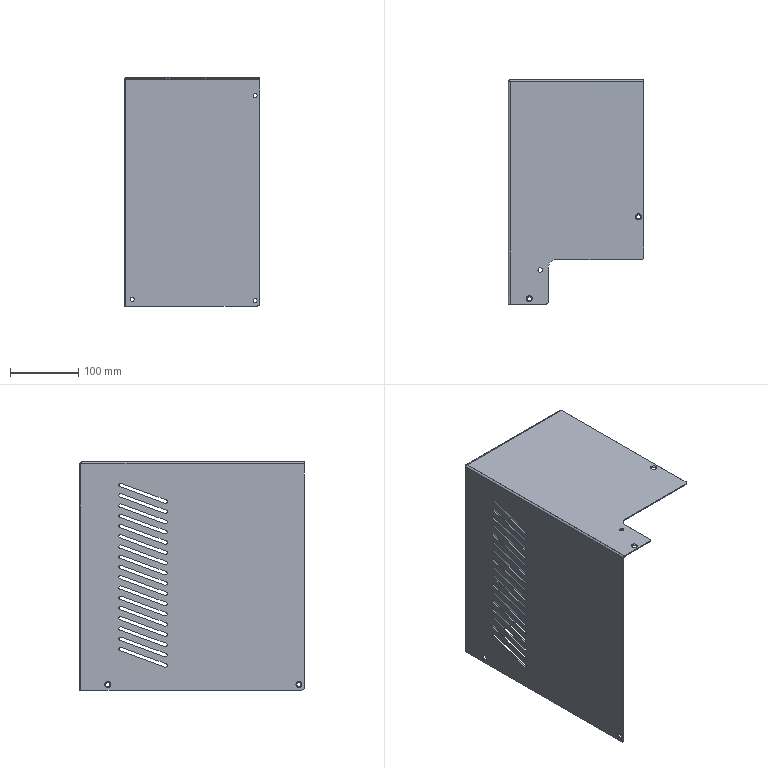Part | SolidWorks | features MirrorStock 1 | 1 solid | 130 faces | box 199 x 329 x 334 mm | volume 335353 mm3 | cylinder 62 | plane 52 | cone 14 | spline 2 | commonest cylinder face diameters 5 x51 8 x4 3 x2 6 x2 6.4 x2 22 x1